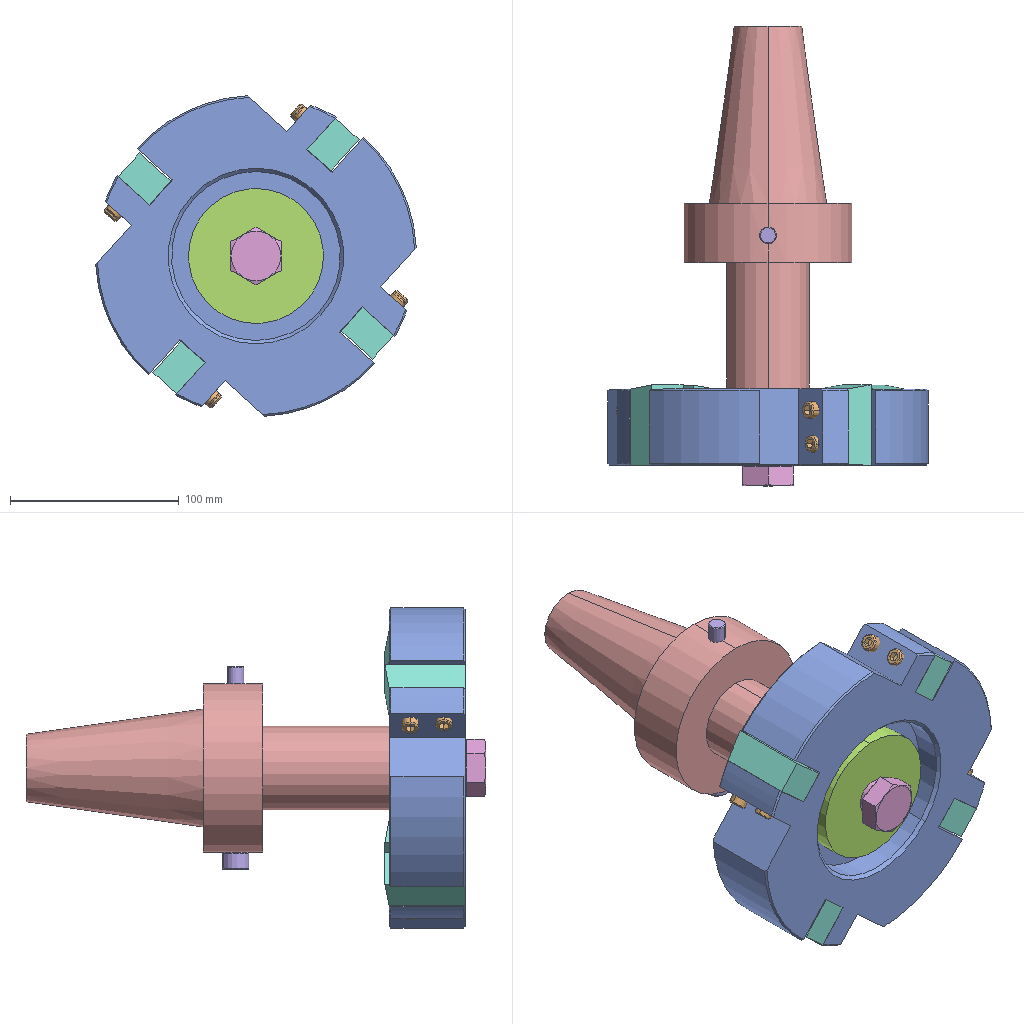Assembly | SolidWorks | 7 different items | 17 placed | box 190 x 272 x 190 mm
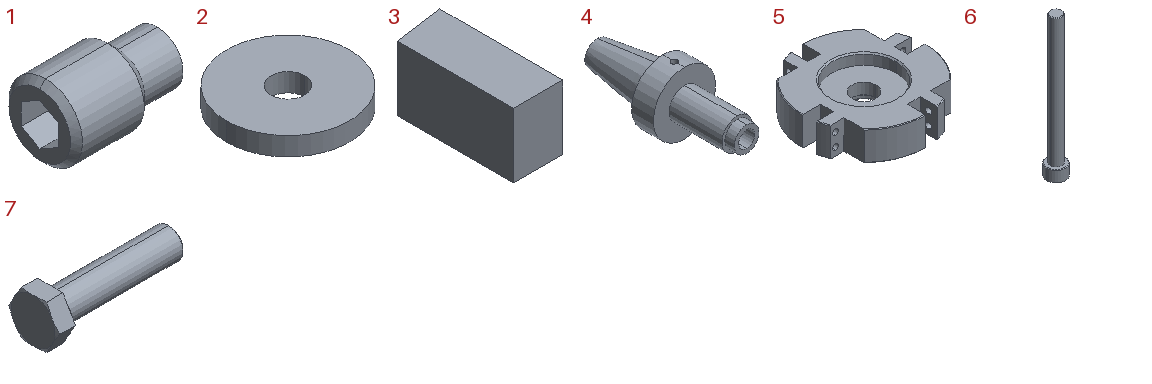Parts list (item | quantity | size | volume | features):
1 | x8 | 16 x 10 x 10 mm | 910.9 mm3 | features RevCut 2, Cut 1, LPattern 1, Revolution 1
2 | x1 | 80 x 80 x 12 mm | 55757 mm3 | features Extrusion 1
3 | x4 | 19 x 47.5 x 25 mm | 21969 mm3 | features Extrusion 1
4 | x1 | 100 x 240 x 100 mm | 634336 mm3 | features ICE 2, 3DProfileFeature 1, HoleWzd 1, RevolutionThin 1
5 | x1 | 190 x 190 x 45 mm | 928420 mm3 | features 3DProfileFeature 5, Chamfer 5, HoleWzd 5, ICE 2, Extrusion 1
6 | x1 | 16 x 16 x 120 mm | 10634 mm3 | features Chamfer 1, Extrusion 1, ICE 1
7 | x1 | 92.28 x 34.26 x 29.67 mm | 34365 mm3 | features RevCut 3, Boss 1, Chamfer 1, Extrusion 1, Fillet 1, LPattern 1
Mates (type | each side: item.copy, entity, surface, feature):
Concentric | 4.1 face cylinder Revolve-Thin1 | 5.1 face cylinder Cut-Extrude1
Coincident | 5.1 face plane Boss-Extrude1 | 3.1 face plane Boss-Extrude1 | 3 times
Coincident | 5.1 face plane Cut-Extrude2 | 2.1 face plane Boss-Extrude1
Concentric | 5.1 face cylinder Cut-Extrude2 | 2.1 face cylinder Boss-Extrude1
Concentric | 5.1 face cylinder Cut-Extrude2 | 7.1 face cylinder BaseBody
Coincident | 5.1 face plane Boss-Extrude1 | 7.1 face plane BaseHead
Concentric | 5.1 face cylinder M10x1.0 Tapped Hole1 | 1.1 face cylinder Base
DistanceDim | 1.1 face plane Base | 5.1 face plane Boss-Extrude1
Concentric | 5.1 face cylinder M10x1.0 Tapped Hole1 | assembly face
Coincident | 5.1 face plane Boss-Extrude1 | assembly face
Concentric | 5.1 face cylinder M10x1.0 Tapped Hole1 | 1.2 face cylinder Base
DistanceDim | 1.2 face plane Base | 5.1 face plane Boss-Extrude1
Coincident | 4.1 face plane Revolve-Thin1 | 5.1 face plane Cut-Extrude1
Concentric | 4.1 face cylinder Cut-Extrude4 | 6.1 face cylinder Boss-Extrude1
Tangent | 4.1 face cylinder Revolve-Thin1 | 6.1 face plane Boss-Extrude2